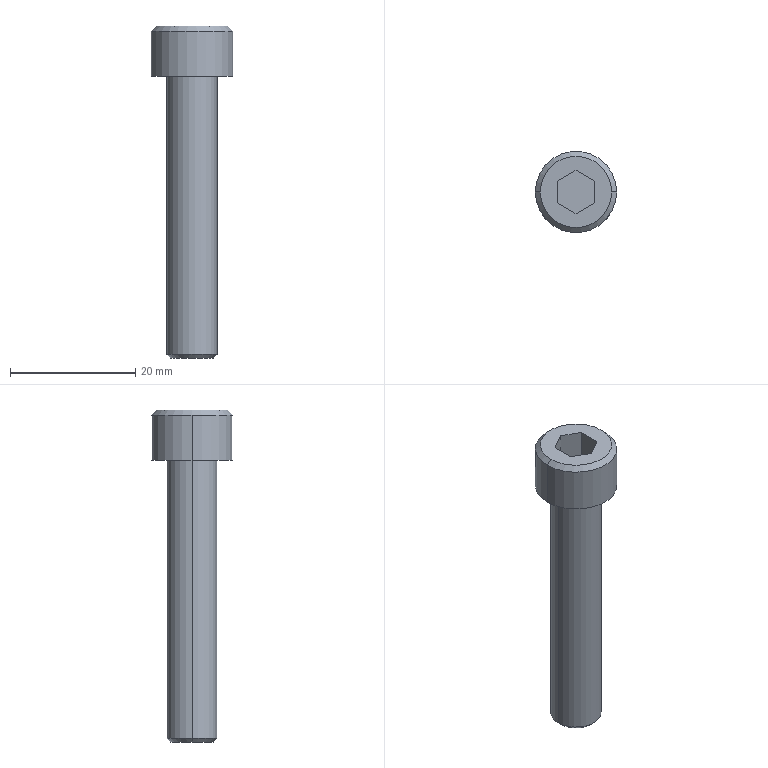Part | Creo | 1 solid | 18 faces | box 13 x 13 x 53 mm | volume 3157 mm3 | plane 10 | cylinder 4 | cone 4 | commonest cylinder face diameters 8 x2 13 x2
STEP:
#1=CARTESIAN_POINT('',(-49.837,-143.386,201.5));
#2=VERTEX_POINT('',#1);
#3=CARTESIAN_POINT('',(-62.837,-143.386,201.5));
#4=VERTEX_POINT('',#3);
#5=CARTESIAN_POINT('',(-56.337,-143.386,201.5));
#6=DIRECTION('',(0.,0.,-1.));
#7=DIRECTION('',(1.,0.,0.));
#8=AXIS2_PLACEMENT_3D('',#5,#6,#7);
#9=CIRCLE('',#8,6.5);
#10=EDGE_CURVE('',#2,#4,#9,.T.);
#11=ORIENTED_EDGE('',*,*,#10,.F.);
#12=CARTESIAN_POINT('',(-56.337,-143.386,201.5));
#13=DIRECTION('',(0.,0.,-1.));
#14=DIRECTION('',(-1.,0.,0.));
#15=AXIS2_PLACEMENT_3D('',#12,#13,#14);
#16=CIRCLE('',#15,6.5);
#17=EDGE_CURVE('',#4,#2,#16,.T.);
#18=ORIENTED_EDGE('',*,*,#17,.F.);
#19=EDGE_LOOP('',(#11,#18));
#20=FACE_OUTER_BOUND('',#19,.F.);
#21=CARTESIAN_POINT('',(-60.337,-143.386,201.5));
#22=VERTEX_POINT('',#21);
#23=CARTESIAN_POINT('',(-52.337,-143.386,201.5));
#24=VERTEX_POINT('',#23);
#25=CARTESIAN_POINT('',(-56.337,-143.386,201.5));
#26=DIRECTION('',(0.,0.,1.));
#27=DIRECTION('',(-1.,0.,0.));
#28=AXIS2_PLACEMENT_3D('',#25,#26,#27);
#29=CIRCLE('',#28,4.);
#30=EDGE_CURVE('',#22,#24,#29,.T.);
#31=ORIENTED_EDGE('',*,*,#30,.F.);
#32=CARTESIAN_POINT('',(-56.337,-143.386,201.5));
#33=DIRECTION('',(0.,0.,1.));
#34=DIRECTION('',(1.,0.,0.));
#35=AXIS2_PLACEMENT_3D('',#32,#33,#34);
#36=CIRCLE('',#35,4.);
#37=EDGE_CURVE('',#24,#22,#36,.T.);
#38=ORIENTED_EDGE('',*,*,#37,.F.);
#39=EDGE_LOOP('',(#31,#38));
#40=FACE_BOUND('',#39,.F.);
#41=CARTESIAN_POINT('',(-56.337,-143.386,201.5));
#42=DIRECTION('',(0.,0.,-1.));
#43=DIRECTION('',(-1.,0.,0.));
#44=AXIS2_PLACEMENT_3D('',#41,#42,#43);
#45=PLANE('',#44);
#46=ADVANCED_FACE('',(#20,#40),#45,.T.);
#47=CARTESIAN_POINT('',(-52.337,-143.386,157.1));
#48=VERTEX_POINT('',#47);
#49=CARTESIAN_POINT('',(-60.337,-143.386,157.1));
#50=VERTEX_POINT('',#49);
#51=CARTESIAN_POINT('',(-56.337,-143.386,157.1));
#52=DIRECTION('',(0.,0.,-1.));
#53=DIRECTION('',(1.,0.,0.));
#54=AXIS2_PLACEMENT_3D('',#51,#52,#53);
#55=CIRCLE('',#54,4.);
#56=EDGE_CURVE('',#48,#50,#55,.T.);
#57=ORIENTED_EDGE('',*,*,#56,.T.);
#58=CARTESIAN_POINT('',(-60.337,-143.386,201.5));
#59=DIRECTION('',(0.,0.,-1.));
#60=VECTOR('',#59,44.4);
#61=LINE('',#58,#60);
#62=EDGE_CURVE('',#22,#50,#61,.T.);
#63=ORIENTED_EDGE('',*,*,#62,.F.);
#64=ORIENTED_EDGE('',*,*,#30,.T.);
#65=CARTESIAN_POINT('',(-52.337,-143.386,201.5));
#66=DIRECTION('',(0.,0.,-1.));
#67=VECTOR('',#66,44.4);
#68=LINE('',#65,#67);
#69=EDGE_CURVE('',#24,#48,#68,.T.);
#70=ORIENTED_EDGE('',*,*,#69,.T.);
#71=EDGE_LOOP('',(#57,#63,#64,#70));
#72=FACE_OUTER_BOUND('',#71,.F.);
#73=CARTESIAN_POINT('',(-56.337,-143.386,210.5));
#74=DIRECTION('',(0.,0.,-1.));
#75=DIRECTION('',(-1.,0.,0.));
#76=AXIS2_PLACEMENT_3D('',#73,#74,#75);
#77=CYLINDRICAL_SURFACE('',#76,4.);
#78=ADVANCED_FACE('',(#72),#77,.T.);
#79=CARTESIAN_POINT('',(-52.937,-143.386,156.5));
#80=VERTEX_POINT('',#79);
#81=CARTESIAN_POINT('',(-59.737,-143.386,156.5));
#82=VERTEX_POINT('',#81);
#83=CARTESIAN_POINT('',(-56.337,-143.386,156.5));
#84=DIRECTION('',(0.,0.,-1.));
#85=DIRECTION('',(1.,0.,0.));
#86=AXIS2_PLACEMENT_3D('',#83,#84,#85);
#87=CIRCLE('',#86,3.4);
#88=EDGE_CURVE('',#80,#82,#87,.T.);
#89=ORIENTED_EDGE('',*,*,#88,.T.);
#90=CARTESIAN_POINT('',(-59.737,-143.386,156.5));
#91=DIRECTION('',(-0.7071,0.,0.7071));
#92=VECTOR('',#91,0.8485);
#93=LINE('',#90,#92);
#94=EDGE_CURVE('',#82,#50,#93,.T.);
#95=ORIENTED_EDGE('',*,*,#94,.T.);
#96=ORIENTED_EDGE('',*,*,#56,.F.);
#97=CARTESIAN_POINT('',(-52.937,-143.386,156.5));
#98=DIRECTION('',(0.7071,0.,0.7071));
#99=VECTOR('',#98,0.8485);
#100=LINE('',#97,#99);
#101=EDGE_CURVE('',#80,#48,#100,.T.);
#102=ORIENTED_EDGE('',*,*,#101,.F.);
#103=EDGE_LOOP('',(#89,#95,#96,#102));
#104=FACE_OUTER_BOUND('',#103,.F.);
#105=CARTESIAN_POINT('',(-56.337,-143.386,156.8));
#106=DIRECTION('',(0.,0.,1.));
#107=DIRECTION('',(1.,0.,0.));
#108=AXIS2_PLACEMENT_3D('',#105,#106,#107);
#109=CONICAL_SURFACE('',#108,3.7,45.);
#110=ADVANCED_FACE('',(#104),#109,.T.);
#111=CARTESIAN_POINT('',(-56.337,-143.386,156.5));
#112=DIRECTION('',(0.,0.,-1.));
#113=DIRECTION('',(-1.,0.,0.));
#114=AXIS2_PLACEMENT_3D('',#111,#112,#113);
#115=CIRCLE('',#114,3.4);
#116=EDGE_CURVE('',#82,#80,#115,.T.);
#117=ORIENTED_EDGE('',*,*,#116,.F.);
#118=ORIENTED_EDGE('',*,*,#88,.F.);
#119=EDGE_LOOP('',(#117,#118));
#120=FACE_OUTER_BOUND('',#119,.F.);
#121=CARTESIAN_POINT('',(-56.337,-143.386,156.5));
#122=DIRECTION('',(0.,0.,-1.));
#123=DIRECTION('',(-1.,0.,0.));
#124=AXIS2_PLACEMENT_3D('',#121,#122,#123);
#125=PLANE('',#124);
#126=ADVANCED_FACE('',(#120),#125,.T.);
#127=ORIENTED_EDGE('',*,*,#116,.T.);
#128=ORIENTED_EDGE('',*,*,#101,.T.);
#129=CARTESIAN_POINT('',(-56.337,-143.386,157.1));
#130=DIRECTION('',(0.,0.,-1.));
#131=DIRECTION('',(-1.,0.,0.));
#132=AXIS2_PLACEMENT_3D('',#129,#130,#131);
#133=CIRCLE('',#132,4.);
#134=EDGE_CURVE('',#50,#48,#133,.T.);
#135=ORIENTED_EDGE('',*,*,#134,.F.);
#136=ORIENTED_EDGE('',*,*,#94,.F.);
#137=EDGE_LOOP('',(#127,#128,#135,#136));
#138=FACE_OUTER_BOUND('',#137,.F.);
#139=CARTESIAN_POINT('',(-56.337,-143.386,156.8));
#140=DIRECTION('',(0.,0.,1.));
#141=DIRECTION('',(1.,0.,0.));
#142=AXIS2_PLACEMENT_3D('',#139,#140,#141);
#143=CONICAL_SURFACE('',#142,3.7,45.);
#144=ADVANCED_FACE('',(#138),#143,.T.);
#145=ORIENTED_EDGE('',*,*,#134,.T.);
#146=ORIENTED_EDGE('',*,*,#69,.F.);
#147=ORIENTED_EDGE('',*,*,#37,.T.);
#148=ORIENTED_EDGE('',*,*,#62,.T.);
#149=EDGE_LOOP('',(#145,#146,#147,#148));
#150=FACE_OUTER_BOUND('',#149,.F.);
#151=CARTESIAN_POINT('',(-56.337,-143.386,210.5));
#152=DIRECTION('',(0.,0.,-1.));
#153=DIRECTION('',(-1.,0.,0.));
#154=AXIS2_PLACEMENT_3D('',#151,#152,#153);
#155=CYLINDRICAL_SURFACE('',#154,4.);
#156=ADVANCED_FACE('',(#150),#155,.T.);
#157=CARTESIAN_POINT('',(-62.837,-143.386,208.7));
#158=VERTEX_POINT('',#157);
#159=CARTESIAN_POINT('',(-49.837,-143.386,208.7));
#160=VERTEX_POINT('',#159);
#161=CARTESIAN_POINT('',(-56.337,-143.386,208.7));
#162=DIRECTION('',(0.,0.,1.));
#163=DIRECTION('',(-1.,0.,0.));
#164=AXIS2_PLACEMENT_3D('',#161,#162,#163);
#165=CIRCLE('',#164,6.5);
#166=EDGE_CURVE('',#158,#160,#165,.T.);
#167=ORIENTED_EDGE('',*,*,#166,.T.);
#168=CARTESIAN_POINT('',(-49.837,-143.386,208.7));
#169=DIRECTION('',(0.,0.,-1.));
#170=VECTOR('',#169,7.2);
#171=LINE('',#168,#170);
#172=EDGE_CURVE('',#160,#2,#171,.T.);
#173=ORIENTED_EDGE('',*,*,#172,.T.);
#174=ORIENTED_EDGE('',*,*,#10,.T.);
#175=CARTESIAN_POINT('',(-62.837,-143.386,208.7));
#176=DIRECTION('',(0.,0.,-1.));
#177=VECTOR('',#176,7.2);
#178=LINE('',#175,#177);
#179=EDGE_CURVE('',#158,#4,#178,.T.);
#180=ORIENTED_EDGE('',*,*,#179,.F.);
#181=EDGE_LOOP('',(#167,#173,#174,#180));
#182=FACE_OUTER_BOUND('',#181,.F.);
#183=CARTESIAN_POINT('',(-56.337,-143.386,210.5));
#184=DIRECTION('',(0.,0.,-1.));
#185=DIRECTION('',(-1.,0.,0.));
#186=AXIS2_PLACEMENT_3D('',#183,#184,#185);
#187=CYLINDRICAL_SURFACE('',#186,6.5);
#188=ADVANCED_FACE('',(#182),#187,.T.);
#189=CARTESIAN_POINT('',(-62.037,-143.386,209.5));
#190=VERTEX_POINT('',#189);
#191=CARTESIAN_POINT('',(-50.637,-143.386,209.5));
#192=VERTEX_POINT('',#191);
#193=CARTESIAN_POINT('',(-56.337,-143.386,209.5));
#194=DIRECTION('',(0.,0.,1.));
#195=DIRECTION('',(-1.,0.,0.));
#196=AXIS2_PLACEMENT_3D('',#193,#194,#195);
#197=CIRCLE('',#196,5.7);
#198=EDGE_CURVE('',#190,#192,#197,.T.);
#199=ORIENTED_EDGE('',*,*,#198,.T.);
#200=CARTESIAN_POINT('',(-50.637,-143.386,209.5));
#201=DIRECTION('',(0.7071,0.,-0.7071));
#202=VECTOR('',#201,1.131);
#203=LINE('',#200,#202);
#204=EDGE_CURVE('',#192,#160,#203,.T.);
#205=ORIENTED_EDGE('',*,*,#204,.T.);
#206=ORIENTED_EDGE('',*,*,#166,.F.);
#207=CARTESIAN_POINT('',(-62.037,-143.386,209.5));
#208=DIRECTION('',(-0.7071,0.,-0.7071));
#209=VECTOR('',#208,1.131);
#210=LINE('',#207,#209);
#211=EDGE_CURVE('',#190,#158,#210,.T.);
#212=ORIENTED_EDGE('',*,*,#211,.F.);
#213=EDGE_LOOP('',(#199,#205,#206,#212));
#214=FACE_OUTER_BOUND('',#213,.F.);
#215=CARTESIAN_POINT('',(-56.337,-143.386,209.1));
#216=DIRECTION('',(0.,0.,-1.));
#217=DIRECTION('',(-1.,0.,0.));
#218=AXIS2_PLACEMENT_3D('',#215,#216,#217);
#219=CONICAL_SURFACE('',#218,6.1,45.);
#220=ADVANCED_FACE('',(#214),#219,.T.);
#221=ORIENTED_EDGE('',*,*,#198,.F.);
#222=CARTESIAN_POINT('',(-56.337,-143.386,209.5));
#223=DIRECTION('',(0.,0.,1.));
#224=DIRECTION('',(1.,0.,0.));
#225=AXIS2_PLACEMENT_3D('',#222,#223,#224);
#226=CIRCLE('',#225,5.7);
#227=EDGE_CURVE('',#192,#190,#226,.T.);
#228=ORIENTED_EDGE('',*,*,#227,.F.);
#229=EDGE_LOOP('',(#221,#228));
#230=FACE_OUTER_BOUND('',#229,.F.);
#231=CARTESIAN_POINT('',(-53.337,-145.118,209.5));
#232=VERTEX_POINT('',#231);
#233=CARTESIAN_POINT('',(-56.337,-146.85,209.5));
#234=VERTEX_POINT('',#233);
#235=CARTESIAN_POINT('',(-53.337,-145.118,209.5));
#236=DIRECTION('',(-0.866,-0.5,0.));
#237=VECTOR('',#236,3.464);
#238=LINE('',#235,#237);
#239=EDGE_CURVE('',#232,#234,#238,.T.);
#240=ORIENTED_EDGE('',*,*,#239,.F.);
#241=CARTESIAN_POINT('',(-53.337,-141.654,209.5));
#242=VERTEX_POINT('',#241);
#243=CARTESIAN_POINT('',(-53.337,-141.654,209.5));
#244=DIRECTION('',(0.,-1.,0.));
#245=VECTOR('',#244,3.464);
#246=LINE('',#243,#245);
#247=EDGE_CURVE('',#242,#232,#246,.T.);
#248=ORIENTED_EDGE('',*,*,#247,.F.);
#249=CARTESIAN_POINT('',(-56.337,-139.922,209.5));
#250=VERTEX_POINT('',#249);
#251=CARTESIAN_POINT('',(-56.337,-139.922,209.5));
#252=DIRECTION('',(0.866,-0.5,0.));
#253=VECTOR('',#252,3.464);
#254=LINE('',#251,#253);
#255=EDGE_CURVE('',#250,#242,#254,.T.);
#256=ORIENTED_EDGE('',*,*,#255,.F.);
#257=CARTESIAN_POINT('',(-59.337,-141.654,209.5));
#258=VERTEX_POINT('',#257);
#259=CARTESIAN_POINT('',(-59.337,-141.654,209.5));
#260=DIRECTION('',(0.866,0.5,0.));
#261=VECTOR('',#260,3.464);
#262=LINE('',#259,#261);
#263=EDGE_CURVE('',#258,#250,#262,.T.);
#264=ORIENTED_EDGE('',*,*,#263,.F.);
#265=CARTESIAN_POINT('',(-59.337,-145.118,209.5));
#266=VERTEX_POINT('',#265);
#267=CARTESIAN_POINT('',(-59.337,-145.118,209.5));
#268=DIRECTION('',(0.,1.,0.));
#269=VECTOR('',#268,3.464);
#270=LINE('',#267,#269);
#271=EDGE_CURVE('',#266,#258,#270,.T.);
#272=ORIENTED_EDGE('',*,*,#271,.F.);
#273=CARTESIAN_POINT('',(-56.337,-146.85,209.5));
#274=DIRECTION('',(-0.866,0.5,0.));
#275=VECTOR('',#274,3.464);
#276=LINE('',#273,#275);
#277=EDGE_CURVE('',#234,#266,#276,.T.);
#278=ORIENTED_EDGE('',*,*,#277,.F.);
#279=EDGE_LOOP('',(#240,#248,#256,#264,#272,#278));
#280=FACE_BOUND('',#279,.F.);
#281=CARTESIAN_POINT('',(-56.337,-143.386,209.5));
#282=DIRECTION('',(0.,0.,-1.));
#283=DIRECTION('',(-1.,0.,0.));
#284=AXIS2_PLACEMENT_3D('',#281,#282,#283);
#285=PLANE('',#284);
#286=ADVANCED_FACE('',(#230,#280),#285,.F.);
#287=ORIENTED_EDGE('',*,*,#227,.T.);
#288=ORIENTED_EDGE('',*,*,#211,.T.);
#289=CARTESIAN_POINT('',(-56.337,-143.386,208.7));
#290=DIRECTION('',(0.,0.,1.));
#291=DIRECTION('',(1.,0.,0.));
#292=AXIS2_PLACEMENT_3D('',#289,#290,#291);
#293=CIRCLE('',#292,6.5);
#294=EDGE_CURVE('',#160,#158,#293,.T.);
#295=ORIENTED_EDGE('',*,*,#294,.F.);
#296=ORIENTED_EDGE('',*,*,#204,.F.);
#297=EDGE_LOOP('',(#287,#288,#295,#296));
#298=FACE_OUTER_BOUND('',#297,.F.);
#299=CARTESIAN_POINT('',(-56.337,-143.386,209.1));
#300=DIRECTION('',(0.,0.,-1.));
#301=DIRECTION('',(-1.,0.,0.));
#302=AXIS2_PLACEMENT_3D('',#299,#300,#301);
#303=CONICAL_SURFACE('',#302,6.1,45.);
#304=ADVANCED_FACE('',(#298),#303,.T.);
#305=ORIENTED_EDGE('',*,*,#294,.T.);
#306=ORIENTED_EDGE('',*,*,#179,.T.);
#307=ORIENTED_EDGE('',*,*,#17,.T.);
#308=ORIENTED_EDGE('',*,*,#172,.F.);
#309=EDGE_LOOP('',(#305,#306,#307,#308));
#310=FACE_OUTER_BOUND('',#309,.F.);
#311=CARTESIAN_POINT('',(-56.337,-143.386,210.5));
#312=DIRECTION('',(0.,0.,-1.));
#313=DIRECTION('',(-1.,0.,0.));
#314=AXIS2_PLACEMENT_3D('',#311,#312,#313);
#315=CYLINDRICAL_SURFACE('',#314,6.5);
#316=ADVANCED_FACE('',(#310),#315,.T.);
#317=ORIENTED_EDGE('',*,*,#239,.T.);
#318=CARTESIAN_POINT('',(-56.337,-146.85,204.7));
#319=VERTEX_POINT('',#318);
#320=CARTESIAN_POINT('',(-56.337,-146.85,209.5));
#321=DIRECTION('',(0.,0.,-1.));
#322=VECTOR('',#321,4.8);
#323=LINE('',#320,#322);
#324=EDGE_CURVE('',#234,#319,#323,.T.);
#325=ORIENTED_EDGE('',*,*,#324,.T.);
#326=CARTESIAN_POINT('',(-53.337,-145.118,204.7));
#327=VERTEX_POINT('',#326);
#328=CARTESIAN_POINT('',(-56.337,-146.85,204.7));
#329=DIRECTION('',(0.866,0.5,0.));
#330=VECTOR('',#329,3.464);
#331=LINE('',#328,#330);
#332=EDGE_CURVE('',#319,#327,#331,.T.);
#333=ORIENTED_EDGE('',*,*,#332,.T.);
#334=CARTESIAN_POINT('',(-53.337,-145.118,209.5));
#335=DIRECTION('',(0.,0.,-1.));
#336=VECTOR('',#335,4.8);
#337=LINE('',#334,#336);
#338=EDGE_CURVE('',#232,#327,#337,.T.);
#339=ORIENTED_EDGE('',*,*,#338,.F.);
#340=EDGE_LOOP('',(#317,#325,#333,#339));
#341=FACE_OUTER_BOUND('',#340,.F.);
#342=CARTESIAN_POINT('',(-56.337,-146.85,204.7));
#343=DIRECTION('',(0.5,-0.866,0.));
#344=DIRECTION('',(0.866,0.5,0.));
#345=AXIS2_PLACEMENT_3D('',#342,#343,#344);
#346=PLANE('',#345);
#347=ADVANCED_FACE('',(#341),#346,.F.);
#348=ORIENTED_EDGE('',*,*,#277,.T.);
#349=CARTESIAN_POINT('',(-59.337,-145.118,204.7));
#350=VERTEX_POINT('',#349);
#351=CARTESIAN_POINT('',(-59.337,-145.118,209.5));
#352=DIRECTION('',(0.,0.,-1.));
#353=VECTOR('',#352,4.8);
#354=LINE('',#351,#353);
#355=EDGE_CURVE('',#266,#350,#354,.T.);
#356=ORIENTED_EDGE('',*,*,#355,.T.);
#357=CARTESIAN_POINT('',(-59.337,-145.118,204.7));
#358=DIRECTION('',(0.866,-0.5,0.));
#359=VECTOR('',#358,3.464);
#360=LINE('',#357,#359);
#361=EDGE_CURVE('',#350,#319,#360,.T.);
#362=ORIENTED_EDGE('',*,*,#361,.T.);
#363=ORIENTED_EDGE('',*,*,#324,.F.);
#364=EDGE_LOOP('',(#348,#356,#362,#363));
#365=FACE_OUTER_BOUND('',#364,.F.);
#366=CARTESIAN_POINT('',(-59.337,-145.118,204.7));
#367=DIRECTION('',(-0.5,-0.866,0.));
#368=DIRECTION('',(0.866,-0.5,0.));
#369=AXIS2_PLACEMENT_3D('',#366,#367,#368);
#370=PLANE('',#369);
#371=ADVANCED_FACE('',(#365),#370,.F.);
#372=ORIENTED_EDGE('',*,*,#271,.T.);
#373=CARTESIAN_POINT('',(-59.337,-141.654,204.7));
#374=VERTEX_POINT('',#373);
#375=CARTESIAN_POINT('',(-59.337,-141.654,209.5));
#376=DIRECTION('',(0.,0.,-1.));
#377=VECTOR('',#376,4.8);
#378=LINE('',#375,#377);
#379=EDGE_CURVE('',#258,#374,#378,.T.);
#380=ORIENTED_EDGE('',*,*,#379,.T.);
#381=CARTESIAN_POINT('',(-59.337,-145.118,204.7));
#382=DIRECTION('',(0.,1.,0.));
#383=VECTOR('',#382,3.464);
#384=LINE('',#381,#383);
#385=EDGE_CURVE('',#350,#374,#384,.T.);
#386=ORIENTED_EDGE('',*,*,#385,.F.);
#387=ORIENTED_EDGE('',*,*,#355,.F.);
#388=EDGE_LOOP('',(#372,#380,#386,#387));
#389=FACE_OUTER_BOUND('',#388,.F.);
#390=CARTESIAN_POINT('',(-59.337,-141.654,204.7));
#391=DIRECTION('',(-1.,0.,0.));
#392=DIRECTION('',(0.,0.,1.));
#393=AXIS2_PLACEMENT_3D('',#390,#391,#392);
#394=PLANE('',#393);
#395=ADVANCED_FACE('',(#389),#394,.F.);
#396=ORIENTED_EDGE('',*,*,#263,.T.);
#397=CARTESIAN_POINT('',(-56.337,-139.922,204.7));
#398=VERTEX_POINT('',#397);
#399=CARTESIAN_POINT('',(-56.337,-139.922,209.5));
#400=DIRECTION('',(0.,0.,-1.));
#401=VECTOR('',#400,4.8);
#402=LINE('',#399,#401);
#403=EDGE_CURVE('',#250,#398,#402,.T.);
#404=ORIENTED_EDGE('',*,*,#403,.T.);
#405=CARTESIAN_POINT('',(-56.337,-139.922,204.7));
#406=DIRECTION('',(-0.866,-0.5,0.));
#407=VECTOR('',#406,3.464);
#408=LINE('',#405,#407);
#409=EDGE_CURVE('',#398,#374,#408,.T.);
#410=ORIENTED_EDGE('',*,*,#409,.T.);
#411=ORIENTED_EDGE('',*,*,#379,.F.);
#412=EDGE_LOOP('',(#396,#404,#410,#411));
#413=FACE_OUTER_BOUND('',#412,.F.);
#414=CARTESIAN_POINT('',(-56.337,-139.922,204.7));
#415=DIRECTION('',(-0.5,0.866,0.));
#416=DIRECTION('',(-0.866,-0.5,0.));
#417=AXIS2_PLACEMENT_3D('',#414,#415,#416);
#418=PLANE('',#417);
#419=ADVANCED_FACE('',(#413),#418,.F.);
#420=ORIENTED_EDGE('',*,*,#255,.T.);
#421=CARTESIAN_POINT('',(-53.337,-141.654,204.7));
#422=VERTEX_POINT('',#421);
#423=CARTESIAN_POINT('',(-53.337,-141.654,209.5));
#424=DIRECTION('',(0.,0.,-1.));
#425=VECTOR('',#424,4.8);
#426=LINE('',#423,#425);
#427=EDGE_CURVE('',#242,#422,#426,.T.);
#428=ORIENTED_EDGE('',*,*,#427,.T.);
#429=CARTESIAN_POINT('',(-53.337,-141.654,204.7));
#430=DIRECTION('',(-0.866,0.5,0.));
#431=VECTOR('',#430,3.464);
#432=LINE('',#429,#431);
#433=EDGE_CURVE('',#422,#398,#432,.T.);
#434=ORIENTED_EDGE('',*,*,#433,.T.);
#435=ORIENTED_EDGE('',*,*,#403,.F.);
#436=EDGE_LOOP('',(#420,#428,#434,#435));
#437=FACE_OUTER_BOUND('',#436,.F.);
#438=CARTESIAN_POINT('',(-53.337,-141.654,204.7));
#439=DIRECTION('',(0.5,0.866,0.));
#440=DIRECTION('',(-0.866,0.5,0.));
#441=AXIS2_PLACEMENT_3D('',#438,#439,#440);
#442=PLANE('',#441);
#443=ADVANCED_FACE('',(#437),#442,.F.);
#444=ORIENTED_EDGE('',*,*,#247,.T.);
#445=ORIENTED_EDGE('',*,*,#338,.T.);
#446=CARTESIAN_POINT('',(-53.337,-141.654,204.7));
#447=DIRECTION('',(0.,-1.,0.));
#448=VECTOR('',#447,3.464);
#449=LINE('',#446,#448);
#450=EDGE_CURVE('',#422,#327,#449,.T.);
#451=ORIENTED_EDGE('',*,*,#450,.F.);
#452=ORIENTED_EDGE('',*,*,#427,.F.);
#453=EDGE_LOOP('',(#444,#445,#451,#452));
#454=FACE_OUTER_BOUND('',#453,.F.);
#455=CARTESIAN_POINT('',(-53.337,-145.118,204.7));
#456=DIRECTION('',(1.,0.,0.));
#457=DIRECTION('',(0.,0.,-1.));
#458=AXIS2_PLACEMENT_3D('',#455,#456,#457);
#459=PLANE('',#458);
#460=ADVANCED_FACE('',(#454),#459,.F.);
#461=ORIENTED_EDGE('',*,*,#361,.F.);
#462=ORIENTED_EDGE('',*,*,#385,.T.);
#463=ORIENTED_EDGE('',*,*,#409,.F.);
#464=ORIENTED_EDGE('',*,*,#433,.F.);
#465=ORIENTED_EDGE('',*,*,#450,.T.);
#466=ORIENTED_EDGE('',*,*,#332,.F.);
#467=EDGE_LOOP('',(#461,#462,#463,#464,#465,#466));
#468=FACE_OUTER_BOUND('',#467,.F.);
#469=CARTESIAN_POINT('',(-56.337,-146.85,204.7));
#470=DIRECTION('',(0.,0.,1.));
#471=DIRECTION('',(1.,0.,0.));
#472=AXIS2_PLACEMENT_3D('',#469,#470,#471);
#473=PLANE('',#472);
#474=ADVANCED_FACE('',(#468),#473,.T.);
#475=CLOSED_SHELL('',(#46,#78,#110,#126,#144,#156,#188,#220,#286,#304,#316,#347,#371,#395,#419,#443,#460,#474));
#476=MANIFOLD_SOLID_BREP('',#475);
#477=(LENGTH_UNIT()NAMED_UNIT(*)SI_UNIT(.MILLI.,.METRE.));
#478=UNCERTAINTY_MEASURE_WITH_UNIT(LENGTH_MEASURE(0.00561),#477,'','');
#479=(NAMED_UNIT(*)PLANE_ANGLE_UNIT()SI_UNIT($,.RADIAN.));
#480=PLANE_ANGLE_MEASURE_WITH_UNIT(PLANE_ANGLE_MEASURE(0.01745),#479);
#481=(CONVERSION_BASED_UNIT('DEGREE',#480)NAMED_UNIT(*)PLANE_ANGLE_UNIT());
#482=(NAMED_UNIT(*)SI_UNIT($,.STERADIAN.)SOLID_ANGLE_UNIT());
#483=(GEOMETRIC_REPRESENTATION_CONTEXT(3)GLOBAL_UNCERTAINTY_ASSIGNED_CONTEXT((#478))GLOBAL_UNIT_ASSIGNED_CONTEXT((#477,#481,#482))REPRESENTATION_CONTEXT('',''));
#484=ADVANCED_BREP_SHAPE_REPRESENTATION('',(#476),#483);